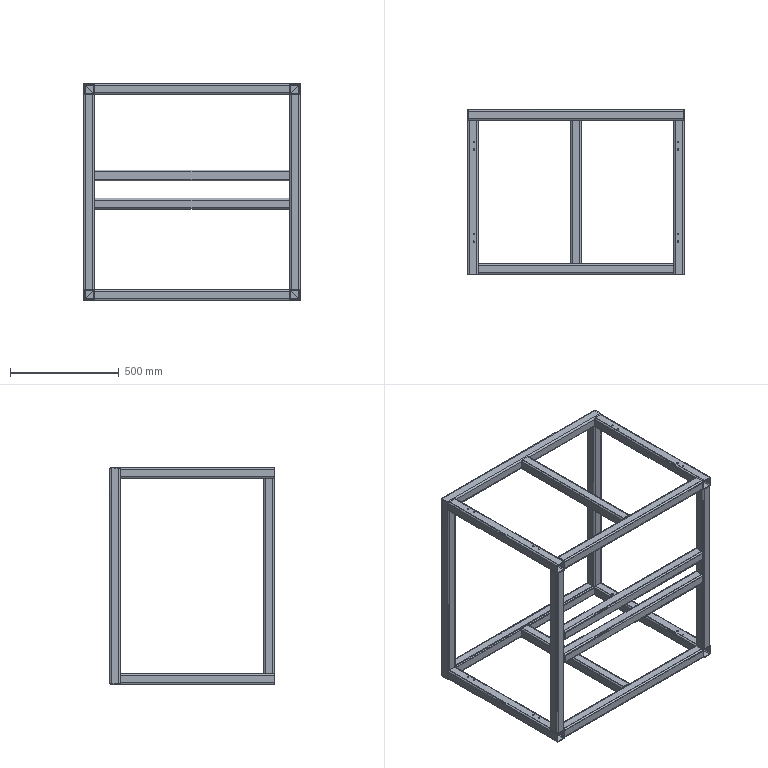Part | SolidWorks | features BaseBody 16 | 16 solids | 352 faces | box 1000 x 760 x 1000 mm | volume 9275053 mm3 | cylinder 192 | plane 160 | commonest cylinder face diameters 6.8 x64 8 x64 16 x64